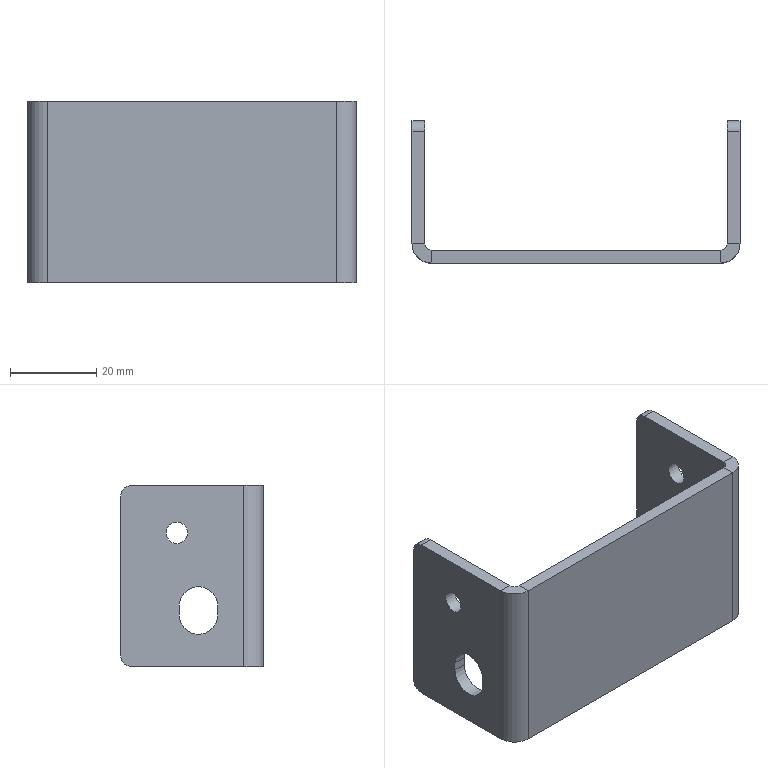Part | STEP file | 5091402 | 1 solid | 36 faces | box 76 x 33 x 42 mm | volume 16188 mm3 | plane 22 | cylinder 14 | commonest cylinder face diameters 5 x6 9 x6 3 x2